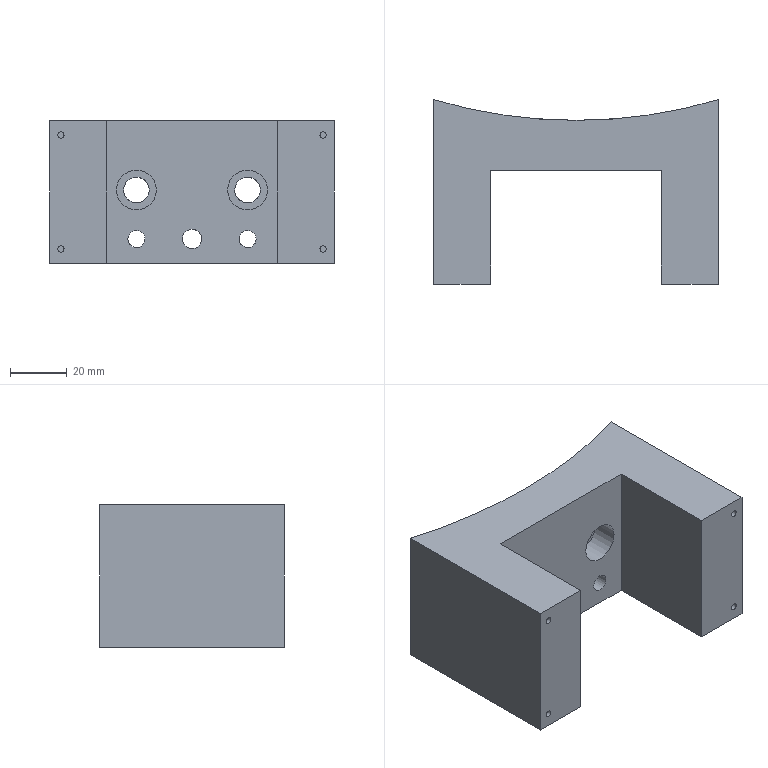Part | NX | 1 solid | 27 faces | box 100 x 64.77 x 50 mm | volume 173660 mm3 | plane 15 | cylinder 12 | commonest cylinder face diameters 2.2 x4 6 x2 9 x2 14 x2 6.8 x1 351 x1
STEP:
#1=CARTESIAN_POINT('',(-50.,32.385,0.));
#2=VERTEX_POINT('',#1);
#3=CARTESIAN_POINT('',(-50.,-32.385,0.));
#4=VERTEX_POINT('',#3);
#5=CARTESIAN_POINT('',(-50.,32.385,0.));
#6=DIRECTION('',(0.,-1.,0.));
#7=VECTOR('',#6,1000.);
#8=LINE('',#5,#7);
#9=EDGE_CURVE('',#2,#4,#8,.T.);
#10=ORIENTED_EDGE('',*,*,#9,.F.);
#11=CARTESIAN_POINT('',(-50.,32.385,-50.));
#12=VERTEX_POINT('',#11);
#13=CARTESIAN_POINT('',(-50.,32.385,-50.));
#14=DIRECTION('',(0.,0.,1.));
#15=VECTOR('',#14,1000.);
#16=LINE('',#13,#15);
#17=EDGE_CURVE('',#12,#2,#16,.T.);
#18=ORIENTED_EDGE('',*,*,#17,.F.);
#19=CARTESIAN_POINT('',(-50.,-32.385,-50.));
#20=VERTEX_POINT('',#19);
#21=CARTESIAN_POINT('',(-50.,32.385,-50.));
#22=DIRECTION('',(0.,-1.,0.));
#23=VECTOR('',#22,1000.);
#24=LINE('',#21,#23);
#25=EDGE_CURVE('',#12,#20,#24,.T.);
#26=ORIENTED_EDGE('',*,*,#25,.T.);
#27=CARTESIAN_POINT('',(-50.,-32.385,-50.));
#28=DIRECTION('',(0.,0.,1.));
#29=VECTOR('',#28,1000.);
#30=LINE('',#27,#29);
#31=EDGE_CURVE('',#20,#4,#30,.T.);
#32=ORIENTED_EDGE('',*,*,#31,.T.);
#33=EDGE_LOOP('',(#10,#18,#26,#32));
#34=FACE_BOUND('',#33,.T.);
#35=CARTESIAN_POINT('',(-50.,32.385,-50.));
#36=DIRECTION('',(-1.,0.,0.));
#37=DIRECTION('',(0.,-1.,0.));
#38=AXIS2_PLACEMENT_3D('',#35,#36,#37);
#39=PLANE('',#38);
#40=ADVANCED_FACE('',(#34),#39,.T.);
#41=CARTESIAN_POINT('',(-44.9,-32.385,-5.));
#42=VERTEX_POINT('',#41);
#43=CARTESIAN_POINT('',(-46.,-32.385,-5.));
#44=DIRECTION('',(0.,1.,0.));
#45=DIRECTION('',(1.,0.,0.));
#46=AXIS2_PLACEMENT_3D('',#43,#44,#45);
#47=CIRCLE('',#46,1.1);
#48=EDGE_CURVE('',#42,#42,#47,.T.);
#49=ORIENTED_EDGE('',*,*,#48,.T.);
#50=EDGE_LOOP('',(#49));
#51=FACE_BOUND('',#50,.T.);
#52=CARTESIAN_POINT('',(-44.9,-32.385,-45.));
#53=VERTEX_POINT('',#52);
#54=CARTESIAN_POINT('',(-46.,-32.385,-45.));
#55=DIRECTION('',(0.,1.,0.));
#56=DIRECTION('',(1.,0.,0.));
#57=AXIS2_PLACEMENT_3D('',#54,#55,#56);
#58=CIRCLE('',#57,1.1);
#59=EDGE_CURVE('',#53,#53,#58,.T.);
#60=ORIENTED_EDGE('',*,*,#59,.T.);
#61=EDGE_LOOP('',(#60));
#62=FACE_BOUND('',#61,.T.);
#63=CARTESIAN_POINT('',(-30.,-32.385,0.));
#64=VERTEX_POINT('',#63);
#65=CARTESIAN_POINT('',(-50.,-32.385,0.));
#66=DIRECTION('',(1.,0.,0.));
#67=VECTOR('',#66,1000.);
#68=LINE('',#65,#67);
#69=EDGE_CURVE('',#4,#64,#68,.T.);
#70=ORIENTED_EDGE('',*,*,#69,.F.);
#71=ORIENTED_EDGE('',*,*,#31,.F.);
#72=CARTESIAN_POINT('',(-30.,-32.385,-50.));
#73=VERTEX_POINT('',#72);
#74=CARTESIAN_POINT('',(-50.,-32.385,-50.));
#75=DIRECTION('',(1.,0.,0.));
#76=VECTOR('',#75,1000.);
#77=LINE('',#74,#76);
#78=EDGE_CURVE('',#20,#73,#77,.T.);
#79=ORIENTED_EDGE('',*,*,#78,.T.);
#80=CARTESIAN_POINT('',(-30.,-32.385,-50.));
#81=DIRECTION('',(0.,0.,1.));
#82=VECTOR('',#81,1000.);
#83=LINE('',#80,#82);
#84=EDGE_CURVE('',#73,#64,#83,.T.);
#85=ORIENTED_EDGE('',*,*,#84,.T.);
#86=EDGE_LOOP('',(#70,#71,#79,#85));
#87=FACE_BOUND('',#86,.T.);
#88=CARTESIAN_POINT('',(-50.,-32.385,-50.));
#89=DIRECTION('',(0.,-1.,0.));
#90=DIRECTION('',(0.,0.,-1.));
#91=AXIS2_PLACEMENT_3D('',#88,#89,#90);
#92=PLANE('',#91);
#93=ADVANCED_FACE('',(#51,#62,#87),#92,.T.);
#94=CARTESIAN_POINT('',(-30.,7.615,0.));
#95=VERTEX_POINT('',#94);
#96=CARTESIAN_POINT('',(-30.,-32.385,0.));
#97=DIRECTION('',(0.,1.,0.));
#98=VECTOR('',#97,1000.);
#99=LINE('',#96,#98);
#100=EDGE_CURVE('',#64,#95,#99,.T.);
#101=ORIENTED_EDGE('',*,*,#100,.F.);
#102=ORIENTED_EDGE('',*,*,#84,.F.);
#103=CARTESIAN_POINT('',(-30.,7.615,-50.));
#104=VERTEX_POINT('',#103);
#105=CARTESIAN_POINT('',(-30.,-32.385,-50.));
#106=DIRECTION('',(0.,1.,0.));
#107=VECTOR('',#106,1000.);
#108=LINE('',#105,#107);
#109=EDGE_CURVE('',#73,#104,#108,.T.);
#110=ORIENTED_EDGE('',*,*,#109,.T.);
#111=CARTESIAN_POINT('',(-30.,7.615,-50.));
#112=DIRECTION('',(0.,0.,1.));
#113=VECTOR('',#112,1000.);
#114=LINE('',#111,#113);
#115=EDGE_CURVE('',#104,#95,#114,.T.);
#116=ORIENTED_EDGE('',*,*,#115,.T.);
#117=EDGE_LOOP('',(#101,#102,#110,#116));
#118=FACE_BOUND('',#117,.T.);
#119=CARTESIAN_POINT('',(-30.,-32.385,-50.));
#120=DIRECTION('',(1.,0.,0.));
#121=DIRECTION('',(0.,1.,0.));
#122=AXIS2_PLACEMENT_3D('',#119,#120,#121);
#123=PLANE('',#122);
#124=ADVANCED_FACE('',(#118),#123,.T.);
#125=CARTESIAN_POINT('',(26.5,7.615,-24.3));
#126=VERTEX_POINT('',#125);
#127=CARTESIAN_POINT('',(19.5,7.615,-24.3));
#128=DIRECTION('',(0.,1.,0.));
#129=DIRECTION('',(1.,0.,0.));
#130=AXIS2_PLACEMENT_3D('',#127,#128,#129);
#131=CIRCLE('',#130,7.);
#132=EDGE_CURVE('',#126,#126,#131,.T.);
#133=ORIENTED_EDGE('',*,*,#132,.T.);
#134=EDGE_LOOP('',(#133));
#135=FACE_BOUND('',#134,.T.);
#136=CARTESIAN_POINT('',(-12.5,7.615,-24.3));
#137=VERTEX_POINT('',#136);
#138=CARTESIAN_POINT('',(-19.5,7.615,-24.3));
#139=DIRECTION('',(0.,1.,0.));
#140=DIRECTION('',(1.,0.,0.));
#141=AXIS2_PLACEMENT_3D('',#138,#139,#140);
#142=CIRCLE('',#141,7.);
#143=EDGE_CURVE('',#137,#137,#142,.T.);
#144=ORIENTED_EDGE('',*,*,#143,.T.);
#145=EDGE_LOOP('',(#144));
#146=FACE_BOUND('',#145,.T.);
#147=CARTESIAN_POINT('',(-16.5,7.615,-41.5));
#148=VERTEX_POINT('',#147);
#149=CARTESIAN_POINT('',(-19.5,7.615,-41.5));
#150=DIRECTION('',(0.,-1.,0.));
#151=DIRECTION('',(1.,0.,0.));
#152=AXIS2_PLACEMENT_3D('',#149,#150,#151);
#153=CIRCLE('',#152,3.);
#154=EDGE_CURVE('',#148,#148,#153,.T.);
#155=ORIENTED_EDGE('',*,*,#154,.F.);
#156=EDGE_LOOP('',(#155));
#157=FACE_BOUND('',#156,.T.);
#158=CARTESIAN_POINT('',(3.4,7.615,-41.5));
#159=VERTEX_POINT('',#158);
#160=CARTESIAN_POINT('',(0.,7.615,-41.5));
#161=DIRECTION('',(0.,-1.,0.));
#162=DIRECTION('',(1.,0.,0.));
#163=AXIS2_PLACEMENT_3D('',#160,#161,#162);
#164=CIRCLE('',#163,3.4);
#165=EDGE_CURVE('',#159,#159,#164,.T.);
#166=ORIENTED_EDGE('',*,*,#165,.F.);
#167=EDGE_LOOP('',(#166));
#168=FACE_BOUND('',#167,.T.);
#169=CARTESIAN_POINT('',(22.5,7.615,-41.5));
#170=VERTEX_POINT('',#169);
#171=CARTESIAN_POINT('',(19.5,7.615,-41.5));
#172=DIRECTION('',(0.,-1.,0.));
#173=DIRECTION('',(1.,0.,0.));
#174=AXIS2_PLACEMENT_3D('',#171,#172,#173);
#175=CIRCLE('',#174,3.);
#176=EDGE_CURVE('',#170,#170,#175,.T.);
#177=ORIENTED_EDGE('',*,*,#176,.F.);
#178=EDGE_LOOP('',(#177));
#179=FACE_BOUND('',#178,.T.);
#180=CARTESIAN_POINT('',(30.,7.615,0.));
#181=VERTEX_POINT('',#180);
#182=CARTESIAN_POINT('',(-30.,7.615,0.));
#183=DIRECTION('',(1.,0.,0.));
#184=VECTOR('',#183,1000.);
#185=LINE('',#182,#184);
#186=EDGE_CURVE('',#95,#181,#185,.T.);
#187=ORIENTED_EDGE('',*,*,#186,.F.);
#188=ORIENTED_EDGE('',*,*,#115,.F.);
#189=CARTESIAN_POINT('',(30.,7.615,-50.));
#190=VERTEX_POINT('',#189);
#191=CARTESIAN_POINT('',(-30.,7.615,-50.));
#192=DIRECTION('',(1.,0.,0.));
#193=VECTOR('',#192,1000.);
#194=LINE('',#191,#193);
#195=EDGE_CURVE('',#104,#190,#194,.T.);
#196=ORIENTED_EDGE('',*,*,#195,.T.);
#197=CARTESIAN_POINT('',(30.,7.615,-50.));
#198=DIRECTION('',(0.,0.,1.));
#199=VECTOR('',#198,1000.);
#200=LINE('',#197,#199);
#201=EDGE_CURVE('',#190,#181,#200,.T.);
#202=ORIENTED_EDGE('',*,*,#201,.T.);
#203=EDGE_LOOP('',(#187,#188,#196,#202));
#204=FACE_BOUND('',#203,.T.);
#205=CARTESIAN_POINT('',(-30.,7.615,-50.));
#206=DIRECTION('',(0.,-1.,0.));
#207=DIRECTION('',(1.,0.,0.));
#208=AXIS2_PLACEMENT_3D('',#205,#206,#207);
#209=PLANE('',#208);
#210=ADVANCED_FACE('',(#135,#146,#157,#168,#179,#204),#209,.T.);
#211=CARTESIAN_POINT('',(30.,-32.385,0.));
#212=VERTEX_POINT('',#211);
#213=CARTESIAN_POINT('',(30.,7.615,0.));
#214=DIRECTION('',(0.,-1.,0.));
#215=VECTOR('',#214,1000.);
#216=LINE('',#213,#215);
#217=EDGE_CURVE('',#181,#212,#216,.T.);
#218=ORIENTED_EDGE('',*,*,#217,.F.);
#219=ORIENTED_EDGE('',*,*,#201,.F.);
#220=CARTESIAN_POINT('',(30.,-32.385,-50.));
#221=VERTEX_POINT('',#220);
#222=CARTESIAN_POINT('',(30.,7.615,-50.));
#223=DIRECTION('',(0.,-1.,0.));
#224=VECTOR('',#223,1000.);
#225=LINE('',#222,#224);
#226=EDGE_CURVE('',#190,#221,#225,.T.);
#227=ORIENTED_EDGE('',*,*,#226,.T.);
#228=CARTESIAN_POINT('',(30.,-32.385,-50.));
#229=DIRECTION('',(0.,0.,1.));
#230=VECTOR('',#229,1000.);
#231=LINE('',#228,#230);
#232=EDGE_CURVE('',#221,#212,#231,.T.);
#233=ORIENTED_EDGE('',*,*,#232,.T.);
#234=EDGE_LOOP('',(#218,#219,#227,#233));
#235=FACE_BOUND('',#234,.T.);
#236=CARTESIAN_POINT('',(30.,7.615,-50.));
#237=DIRECTION('',(-1.,0.,0.));
#238=DIRECTION('',(0.,-1.,0.));
#239=AXIS2_PLACEMENT_3D('',#236,#237,#238);
#240=PLANE('',#239);
#241=ADVANCED_FACE('',(#235),#240,.T.);
#242=CARTESIAN_POINT('',(47.1,-32.385,-45.));
#243=VERTEX_POINT('',#242);
#244=CARTESIAN_POINT('',(46.,-32.385,-45.));
#245=DIRECTION('',(0.,1.,0.));
#246=DIRECTION('',(1.,0.,0.));
#247=AXIS2_PLACEMENT_3D('',#244,#245,#246);
#248=CIRCLE('',#247,1.1);
#249=EDGE_CURVE('',#243,#243,#248,.T.);
#250=ORIENTED_EDGE('',*,*,#249,.T.);
#251=EDGE_LOOP('',(#250));
#252=FACE_BOUND('',#251,.T.);
#253=CARTESIAN_POINT('',(47.1,-32.385,-5.));
#254=VERTEX_POINT('',#253);
#255=CARTESIAN_POINT('',(46.,-32.385,-5.));
#256=DIRECTION('',(0.,1.,0.));
#257=DIRECTION('',(1.,0.,0.));
#258=AXIS2_PLACEMENT_3D('',#255,#256,#257);
#259=CIRCLE('',#258,1.1);
#260=EDGE_CURVE('',#254,#254,#259,.T.);
#261=ORIENTED_EDGE('',*,*,#260,.T.);
#262=EDGE_LOOP('',(#261));
#263=FACE_BOUND('',#262,.T.);
#264=CARTESIAN_POINT('',(50.,-32.385,0.));
#265=VERTEX_POINT('',#264);
#266=CARTESIAN_POINT('',(30.,-32.385,0.));
#267=DIRECTION('',(1.,0.,0.));
#268=VECTOR('',#267,1000.);
#269=LINE('',#266,#268);
#270=EDGE_CURVE('',#212,#265,#269,.T.);
#271=ORIENTED_EDGE('',*,*,#270,.F.);
#272=ORIENTED_EDGE('',*,*,#232,.F.);
#273=CARTESIAN_POINT('',(50.,-32.385,-50.));
#274=VERTEX_POINT('',#273);
#275=CARTESIAN_POINT('',(30.,-32.385,-50.));
#276=DIRECTION('',(1.,0.,0.));
#277=VECTOR('',#276,1000.);
#278=LINE('',#275,#277);
#279=EDGE_CURVE('',#221,#274,#278,.T.);
#280=ORIENTED_EDGE('',*,*,#279,.T.);
#281=CARTESIAN_POINT('',(50.,-32.385,-50.));
#282=DIRECTION('',(0.,0.,1.));
#283=VECTOR('',#282,1000.);
#284=LINE('',#281,#283);
#285=EDGE_CURVE('',#274,#265,#284,.T.);
#286=ORIENTED_EDGE('',*,*,#285,.T.);
#287=EDGE_LOOP('',(#271,#272,#280,#286));
#288=FACE_BOUND('',#287,.T.);
#289=CARTESIAN_POINT('',(30.,-32.385,-50.));
#290=DIRECTION('',(0.,-1.,0.));
#291=DIRECTION('',(0.,0.,-1.));
#292=AXIS2_PLACEMENT_3D('',#289,#290,#291);
#293=PLANE('',#292);
#294=ADVANCED_FACE('',(#252,#263,#288),#293,.T.);
#295=CARTESIAN_POINT('',(50.,32.385,0.));
#296=VERTEX_POINT('',#295);
#297=CARTESIAN_POINT('',(50.,-32.385,0.));
#298=DIRECTION('',(0.,1.,0.));
#299=VECTOR('',#298,1000.);
#300=LINE('',#297,#299);
#301=EDGE_CURVE('',#265,#296,#300,.T.);
#302=ORIENTED_EDGE('',*,*,#301,.F.);
#303=ORIENTED_EDGE('',*,*,#285,.F.);
#304=CARTESIAN_POINT('',(50.,32.385,-50.));
#305=VERTEX_POINT('',#304);
#306=CARTESIAN_POINT('',(50.,-32.385,-50.));
#307=DIRECTION('',(0.,1.,0.));
#308=VECTOR('',#307,1000.);
#309=LINE('',#306,#308);
#310=EDGE_CURVE('',#274,#305,#309,.T.);
#311=ORIENTED_EDGE('',*,*,#310,.T.);
#312=CARTESIAN_POINT('',(50.,32.385,-50.));
#313=DIRECTION('',(0.,0.,1.));
#314=VECTOR('',#313,1000.);
#315=LINE('',#312,#314);
#316=EDGE_CURVE('',#305,#296,#315,.T.);
#317=ORIENTED_EDGE('',*,*,#316,.T.);
#318=EDGE_LOOP('',(#302,#303,#311,#317));
#319=FACE_BOUND('',#318,.T.);
#320=CARTESIAN_POINT('',(50.,-32.385,-50.));
#321=DIRECTION('',(1.,0.,0.));
#322=DIRECTION('',(0.,1.,0.));
#323=AXIS2_PLACEMENT_3D('',#320,#321,#322);
#324=PLANE('',#323);
#325=ADVANCED_FACE('',(#319),#324,.T.);
#326=CARTESIAN_POINT('',(-19.5,26.198,-19.8));
#327=VERTEX_POINT('',#326);
#328=CARTESIAN_POINT('',(-23.019,26.621,-20.766));
#329=CARTESIAN_POINT('',(-19.501,26.184,-19.316));
#330=CARTESIAN_POINT('',(-15.979,25.834,-20.769));
#331=CARTESIAN_POINT('',(-14.51,25.714,-24.301));
#332=CARTESIAN_POINT('',(-15.983,25.834,-27.838));
#333=CARTESIAN_POINT('',(-19.511,26.185,-29.282));
#334=CARTESIAN_POINT('',(-23.016,26.621,-27.833));
#335=CARTESIAN_POINT('',(-24.491,26.83,-24.302));
#336=CARTESIAN_POINT('',(-23.019,26.621,-20.766));
#337=CARTESIAN_POINT('',(-19.501,26.184,-19.316));
#338=CARTESIAN_POINT('',(-15.979,25.834,-20.769));
#339=B_SPLINE_CURVE_WITH_KNOTS('',3,(#328,#329,#330,#331,#332,#333,#334,#335,#336,#337,#338),.UNSPECIFIED.,.T.,.F.,(1,1,1,1,1,1,1,1,1,1,1,1,1,1,1),(-0.01058,-0.007056,-0.003528,0.,0.003528,0.007056,0.01058,0.01411,0.01764,0.02117,0.02469,0.02822,0.03175,0.03528,0.03881),.UNSPECIFIED.);
#340=EDGE_CURVE('',#327,#327,#339,.T.);
#341=ORIENTED_EDGE('',*,*,#340,.F.);
#342=EDGE_LOOP('',(#341));
#343=FACE_BOUND('',#342,.T.);
#344=CARTESIAN_POINT('',(-19.5,26.198,-38.5));
#345=VERTEX_POINT('',#344);
#346=CARTESIAN_POINT('',(-21.846,26.474,-39.145));
#347=CARTESIAN_POINT('',(-19.5,26.192,-38.178));
#348=CARTESIAN_POINT('',(-17.153,25.949,-39.145));
#349=CARTESIAN_POINT('',(-16.173,25.859,-41.499));
#350=CARTESIAN_POINT('',(-17.155,25.949,-43.858));
#351=CARTESIAN_POINT('',(-19.505,26.193,-44.821));
#352=CARTESIAN_POINT('',(-21.844,26.473,-43.857));
#353=CARTESIAN_POINT('',(-22.827,26.603,-41.502));
#354=CARTESIAN_POINT('',(-21.846,26.474,-39.145));
#355=CARTESIAN_POINT('',(-19.5,26.192,-38.178));
#356=CARTESIAN_POINT('',(-17.153,25.949,-39.145));
#357=B_SPLINE_CURVE_WITH_KNOTS('',3,(#346,#347,#348,#349,#350,#351,#352,#353,#354,#355,#356),.UNSPECIFIED.,.T.,.F.,(1,1,1,1,1,1,1,1,1,1,1,1,1,1,1),(-0.007055,-0.004704,-0.002352,0.,0.002352,0.004704,0.007055,0.009407,0.01176,0.01411,0.01646,0.01881,0.02117,0.02352,0.02587),.UNSPECIFIED.);
#358=EDGE_CURVE('',#345,#345,#357,.T.);
#359=ORIENTED_EDGE('',*,*,#358,.F.);
#360=EDGE_LOOP('',(#359));
#361=FACE_BOUND('',#360,.T.);
#362=CARTESIAN_POINT('',(0.,25.112,-38.1));
#363=VERTEX_POINT('',#362);
#364=CARTESIAN_POINT('',(-2.667,25.128,-38.838));
#365=CARTESIAN_POINT('',(0.0006847,25.104,-37.731));
#366=CARTESIAN_POINT('',(2.665,25.128,-38.837));
#367=CARTESIAN_POINT('',(3.767,25.153,-41.497));
#368=CARTESIAN_POINT('',(2.666,25.128,-44.163));
#369=CARTESIAN_POINT('',(0.0004927,25.104,-45.267));
#370=CARTESIAN_POINT('',(-2.661,25.128,-44.167));
#371=CARTESIAN_POINT('',(-3.768,25.153,-41.504));
#372=CARTESIAN_POINT('',(-2.667,25.128,-38.838));
#373=CARTESIAN_POINT('',(0.0006847,25.104,-37.731));
#374=CARTESIAN_POINT('',(2.665,25.128,-38.837));
#375=B_SPLINE_CURVE_WITH_KNOTS('',3,(#364,#365,#366,#367,#368,#369,#370,#371,#372,#373,#374),.UNSPECIFIED.,.T.,.F.,(1,1,1,1,1,1,1,1,1,1,1,1,1,1,1),(-0.007972,-0.005315,-0.002657,0.,0.002657,0.005315,0.007972,0.01063,0.01329,0.01594,0.0186,0.02126,0.02392,0.02657,0.02923),.UNSPECIFIED.);
#376=EDGE_CURVE('',#363,#363,#375,.T.);
#377=ORIENTED_EDGE('',*,*,#376,.F.);
#378=EDGE_LOOP('',(#377));
#379=FACE_BOUND('',#378,.T.);
#380=CARTESIAN_POINT('',(19.5,26.198,-19.8));
#381=VERTEX_POINT('',#380);
#382=CARTESIAN_POINT('',(15.975,25.834,-20.77));
#383=CARTESIAN_POINT('',(19.503,26.184,-19.316));
#384=CARTESIAN_POINT('',(23.014,26.621,-20.765));
#385=CARTESIAN_POINT('',(24.49,26.83,-24.291));
#386=CARTESIAN_POINT('',(23.024,26.622,-27.828));
#387=CARTESIAN_POINT('',(19.512,26.185,-29.282));
#388=CARTESIAN_POINT('',(15.991,25.835,-27.843));
#389=CARTESIAN_POINT('',(14.509,25.714,-24.311));
#390=CARTESIAN_POINT('',(15.975,25.834,-20.77));
#391=CARTESIAN_POINT('',(19.503,26.184,-19.316));
#392=CARTESIAN_POINT('',(23.014,26.621,-20.765));
#393=B_SPLINE_CURVE_WITH_KNOTS('',3,(#382,#383,#384,#385,#386,#387,#388,#389,#390,#391,#392),.UNSPECIFIED.,.T.,.F.,(1,1,1,1,1,1,1,1,1,1,1,1,1,1,1),(-0.01058,-0.007055,-0.003528,0.,0.003528,0.007055,0.01058,0.01411,0.01764,0.02117,0.02469,0.02822,0.03175,0.03528,0.0388),.UNSPECIFIED.);
#394=EDGE_CURVE('',#381,#381,#393,.T.);
#395=ORIENTED_EDGE('',*,*,#394,.F.);
#396=EDGE_LOOP('',(#395));
#397=FACE_BOUND('',#396,.T.);
#398=CARTESIAN_POINT('',(19.5,26.198,-38.5));
#399=VERTEX_POINT('',#398);
#400=CARTESIAN_POINT('',(17.15,25.949,-39.146));
#401=CARTESIAN_POINT('',(19.501,26.192,-38.178));
#402=CARTESIAN_POINT('',(21.844,26.473,-39.144));
#403=CARTESIAN_POINT('',(22.827,26.603,-41.495));
#404=CARTESIAN_POINT('',(21.848,26.474,-43.853));
#405=CARTESIAN_POINT('',(19.505,26.193,-44.821));
#406=CARTESIAN_POINT('',(17.16,25.95,-43.861));
#407=CARTESIAN_POINT('',(16.172,25.859,-41.506));
#408=CARTESIAN_POINT('',(17.15,25.949,-39.146));
#409=CARTESIAN_POINT('',(19.501,26.192,-38.178));
#410=CARTESIAN_POINT('',(21.844,26.473,-39.144));
#411=B_SPLINE_CURVE_WITH_KNOTS('',3,(#400,#401,#402,#403,#404,#405,#406,#407,#408,#409,#410),.UNSPECIFIED.,.T.,.F.,(1,1,1,1,1,1,1,1,1,1,1,1,1,1,1),(-0.007055,-0.004704,-0.002352,0.,0.002352,0.004704,0.007055,0.009407,0.01176,0.01411,0.01646,0.01881,0.02117,0.02352,0.02587),.UNSPECIFIED.);
#412=EDGE_CURVE('',#399,#399,#411,.T.);
#413=ORIENTED_EDGE('',*,*,#412,.F.);
#414=EDGE_LOOP('',(#413));
#415=FACE_BOUND('',#414,.T.);
#416=CARTESIAN_POINT('',(0.,200.612,0.));
#417=DIRECTION('',(0.,0.,-1.));
#418=DIRECTION('',(1.,0.,0.));
#419=AXIS2_PLACEMENT_3D('',#416,#417,#418);
#420=CIRCLE('',#419,175.5);
#421=EDGE_CURVE('',#296,#2,#420,.T.);
#422=ORIENTED_EDGE('',*,*,#421,.F.);
#423=ORIENTED_EDGE('',*,*,#316,.F.);
#424=CARTESIAN_POINT('',(0.,200.612,-50.));
#425=DIRECTION('',(0.,0.,-1.));
#426=DIRECTION('',(1.,0.,0.));
#427=AXIS2_PLACEMENT_3D('',#424,#425,#426);
#428=CIRCLE('',#427,175.5);
#429=EDGE_CURVE('',#305,#12,#428,.T.);
#430=ORIENTED_EDGE('',*,*,#429,.T.);
#431=ORIENTED_EDGE('',*,*,#17,.T.);
#432=EDGE_LOOP('',(#422,#423,#430,#431));
#433=FACE_BOUND('',#432,.T.);
#434=CARTESIAN_POINT('',(0.,200.612,-50.));
#435=DIRECTION('',(0.,0.,1.));
#436=DIRECTION('',(1.,0.,0.));
#437=AXIS2_PLACEMENT_3D('',#434,#435,#436);
#438=CYLINDRICAL_SURFACE('',#437,175.5);
#439=ADVANCED_FACE('',(#343,#361,#379,#397,#415,#433),#438,.F.);
#440=ORIENTED_EDGE('',*,*,#25,.F.);
#441=ORIENTED_EDGE('',*,*,#429,.F.);
#442=ORIENTED_EDGE('',*,*,#310,.F.);
#443=ORIENTED_EDGE('',*,*,#279,.F.);
#444=ORIENTED_EDGE('',*,*,#226,.F.);
#445=ORIENTED_EDGE('',*,*,#195,.F.);
#446=ORIENTED_EDGE('',*,*,#109,.F.);
#447=ORIENTED_EDGE('',*,*,#78,.F.);
#448=EDGE_LOOP('',(#440,#441,#442,#443,#444,#445,#446,#447));
#449=FACE_BOUND('',#448,.T.);
#450=CARTESIAN_POINT('',(0.,200.612,-50.));
#451=DIRECTION('',(0.,0.,-1.));
#452=DIRECTION('',(-1.,0.,0.));
#453=AXIS2_PLACEMENT_3D('',#450,#451,#452);
#454=PLANE('',#453);
#455=ADVANCED_FACE('',(#449),#454,.T.);
#456=ORIENTED_EDGE('',*,*,#9,.T.);
#457=ORIENTED_EDGE('',*,*,#69,.T.);
#458=ORIENTED_EDGE('',*,*,#100,.T.);
#459=ORIENTED_EDGE('',*,*,#186,.T.);
#460=ORIENTED_EDGE('',*,*,#217,.T.);
#461=ORIENTED_EDGE('',*,*,#270,.T.);
#462=ORIENTED_EDGE('',*,*,#301,.T.);
#463=ORIENTED_EDGE('',*,*,#421,.T.);
#464=EDGE_LOOP('',(#456,#457,#458,#459,#460,#461,#462,#463));
#465=FACE_BOUND('',#464,.T.);
#466=CARTESIAN_POINT('',(0.,200.612,0.));
#467=DIRECTION('',(0.,0.,-1.));
#468=DIRECTION('',(-1.,0.,0.));
#469=AXIS2_PLACEMENT_3D('',#466,#467,#468);
#470=PLANE('',#469);
#471=ADVANCED_FACE('',(#465),#470,.F.);
#472=ORIENTED_EDGE('',*,*,#260,.F.);
#473=EDGE_LOOP('',(#472));
#474=FACE_BOUND('',#473,.T.);
#475=CARTESIAN_POINT('',(47.1,-21.385,-5.));
#476=VERTEX_POINT('',#475);
#477=CARTESIAN_POINT('',(46.,-21.385,-5.));
#478=DIRECTION('',(0.,1.,0.));
#479=DIRECTION('',(1.,0.,0.));
#480=AXIS2_PLACEMENT_3D('',#477,#478,#479);
#481=CIRCLE('',#480,1.1);
#482=EDGE_CURVE('',#476,#476,#481,.F.);
#483=ORIENTED_EDGE('',*,*,#482,.F.);
#484=EDGE_LOOP('',(#483));
#485=FACE_BOUND('',#484,.T.);
#486=CARTESIAN_POINT('',(46.,-32.385,-5.));
#487=DIRECTION('',(0.,1.,0.));
#488=DIRECTION('',(0.,0.,1.));
#489=AXIS2_PLACEMENT_3D('',#486,#487,#488);
#490=CYLINDRICAL_SURFACE('',#489,1.1);
#491=ADVANCED_FACE('',(#474,#485),#490,.F.);
#492=ORIENTED_EDGE('',*,*,#482,.T.);
#493=EDGE_LOOP('',(#492));
#494=FACE_BOUND('',#493,.T.);
#495=CARTESIAN_POINT('',(46.,-21.385,-5.));
#496=DIRECTION('',(0.,1.,0.));
#497=DIRECTION('',(0.,0.,1.));
#498=AXIS2_PLACEMENT_3D('',#495,#496,#497);
#499=PLANE('',#498);
#500=ADVANCED_FACE('',(#494),#499,.F.);
#501=ORIENTED_EDGE('',*,*,#249,.F.);
#502=EDGE_LOOP('',(#501));
#503=FACE_BOUND('',#502,.T.);
#504=CARTESIAN_POINT('',(47.1,-21.385,-45.));
#505=VERTEX_POINT('',#504);
#506=CARTESIAN_POINT('',(46.,-21.385,-45.));
#507=DIRECTION('',(0.,1.,0.));
#508=DIRECTION('',(1.,0.,0.));
#509=AXIS2_PLACEMENT_3D('',#506,#507,#508);
#510=CIRCLE('',#509,1.1);
#511=EDGE_CURVE('',#505,#505,#510,.F.);
#512=ORIENTED_EDGE('',*,*,#511,.F.);
#513=EDGE_LOOP('',(#512));
#514=FACE_BOUND('',#513,.T.);
#515=CARTESIAN_POINT('',(46.,-32.385,-45.));
#516=DIRECTION('',(0.,1.,0.));
#517=DIRECTION('',(0.,0.,1.));
#518=AXIS2_PLACEMENT_3D('',#515,#516,#517);
#519=CYLINDRICAL_SURFACE('',#518,1.1);
#520=ADVANCED_FACE('',(#503,#514),#519,.F.);
#521=ORIENTED_EDGE('',*,*,#511,.T.);
#522=EDGE_LOOP('',(#521));
#523=FACE_BOUND('',#522,.T.);
#524=CARTESIAN_POINT('',(46.,-21.385,-45.));
#525=DIRECTION('',(0.,1.,0.));
#526=DIRECTION('',(0.,0.,1.));
#527=AXIS2_PLACEMENT_3D('',#524,#525,#526);
#528=PLANE('',#527);
#529=ADVANCED_FACE('',(#523),#528,.F.);
#530=ORIENTED_EDGE('',*,*,#59,.F.);
#531=EDGE_LOOP('',(#530));
#532=FACE_BOUND('',#531,.T.);
#533=CARTESIAN_POINT('',(-44.9,-21.385,-45.));
#534=VERTEX_POINT('',#533);
#535=CARTESIAN_POINT('',(-46.,-21.385,-45.));
#536=DIRECTION('',(0.,1.,0.));
#537=DIRECTION('',(1.,0.,0.));
#538=AXIS2_PLACEMENT_3D('',#535,#536,#537);
#539=CIRCLE('',#538,1.1);
#540=EDGE_CURVE('',#534,#534,#539,.F.);
#541=ORIENTED_EDGE('',*,*,#540,.F.);
#542=EDGE_LOOP('',(#541));
#543=FACE_BOUND('',#542,.T.);
#544=CARTESIAN_POINT('',(-46.,-32.385,-45.));
#545=DIRECTION('',(0.,1.,0.));
#546=DIRECTION('',(0.,0.,1.));
#547=AXIS2_PLACEMENT_3D('',#544,#545,#546);
#548=CYLINDRICAL_SURFACE('',#547,1.1);
#549=ADVANCED_FACE('',(#532,#543),#548,.F.);
#550=ORIENTED_EDGE('',*,*,#540,.T.);
#551=EDGE_LOOP('',(#550));
#552=FACE_BOUND('',#551,.T.);
#553=CARTESIAN_POINT('',(-46.,-21.385,-45.));
#554=DIRECTION('',(0.,1.,0.));
#555=DIRECTION('',(0.,0.,1.));
#556=AXIS2_PLACEMENT_3D('',#553,#554,#555);
#557=PLANE('',#556);
#558=ADVANCED_FACE('',(#552),#557,.F.);
#559=ORIENTED_EDGE('',*,*,#48,.F.);
#560=EDGE_LOOP('',(#559));
#561=FACE_BOUND('',#560,.T.);
#562=CARTESIAN_POINT('',(-44.9,-21.385,-5.));
#563=VERTEX_POINT('',#562);
#564=CARTESIAN_POINT('',(-46.,-21.385,-5.));
#565=DIRECTION('',(0.,1.,0.));
#566=DIRECTION('',(1.,0.,0.));
#567=AXIS2_PLACEMENT_3D('',#564,#565,#566);
#568=CIRCLE('',#567,1.1);
#569=EDGE_CURVE('',#563,#563,#568,.F.);
#570=ORIENTED_EDGE('',*,*,#569,.F.);
#571=EDGE_LOOP('',(#570));
#572=FACE_BOUND('',#571,.T.);
#573=CARTESIAN_POINT('',(-46.,-32.385,-5.));
#574=DIRECTION('',(0.,1.,0.));
#575=DIRECTION('',(0.,0.,1.));
#576=AXIS2_PLACEMENT_3D('',#573,#574,#575);
#577=CYLINDRICAL_SURFACE('',#576,1.1);
#578=ADVANCED_FACE('',(#561,#572),#577,.F.);
#579=ORIENTED_EDGE('',*,*,#569,.T.);
#580=EDGE_LOOP('',(#579));
#581=FACE_BOUND('',#580,.T.);
#582=CARTESIAN_POINT('',(-46.,-21.385,-5.));
#583=DIRECTION('',(0.,1.,0.));
#584=DIRECTION('',(0.,0.,1.));
#585=AXIS2_PLACEMENT_3D('',#582,#583,#584);
#586=PLANE('',#585);
#587=ADVANCED_FACE('',(#581),#586,.F.);
#588=ORIENTED_EDGE('',*,*,#176,.T.);
#589=EDGE_LOOP('',(#588));
#590=FACE_BOUND('',#589,.T.);
#591=ORIENTED_EDGE('',*,*,#412,.T.);
#592=EDGE_LOOP('',(#591));
#593=FACE_BOUND('',#592,.T.);
#594=CARTESIAN_POINT('',(19.5,-32.385,-41.5));
#595=DIRECTION('',(0.,1.,0.));
#596=DIRECTION('',(0.,0.,1.));
#597=AXIS2_PLACEMENT_3D('',#594,#595,#596);
#598=CYLINDRICAL_SURFACE('',#597,3.);
#599=ADVANCED_FACE('',(#590,#593),#598,.F.);
#600=CARTESIAN_POINT('',(24.,16.615,-24.3));
#601=VERTEX_POINT('',#600);
#602=CARTESIAN_POINT('',(19.5,16.615,-24.3));
#603=DIRECTION('',(0.,1.,0.));
#604=DIRECTION('',(1.,0.,0.));
#605=AXIS2_PLACEMENT_3D('',#602,#603,#604);
#606=CIRCLE('',#605,4.5);
#607=EDGE_CURVE('',#601,#601,#606,.T.);
#608=ORIENTED_EDGE('',*,*,#607,.F.);
#609=EDGE_LOOP('',(#608));
#610=FACE_BOUND('',#609,.T.);
#611=ORIENTED_EDGE('',*,*,#394,.T.);
#612=EDGE_LOOP('',(#611));
#613=FACE_BOUND('',#612,.T.);
#614=CARTESIAN_POINT('',(19.5,-32.385,-24.3));
#615=DIRECTION('',(0.,1.,0.));
#616=DIRECTION('',(0.,0.,1.));
#617=AXIS2_PLACEMENT_3D('',#614,#615,#616);
#618=CYLINDRICAL_SURFACE('',#617,4.5);
#619=ADVANCED_FACE('',(#610,#613),#618,.F.);
#620=ORIENTED_EDGE('',*,*,#165,.T.);
#621=EDGE_LOOP('',(#620));
#622=FACE_BOUND('',#621,.T.);
#623=ORIENTED_EDGE('',*,*,#376,.T.);
#624=EDGE_LOOP('',(#623));
#625=FACE_BOUND('',#624,.T.);
#626=CARTESIAN_POINT('',(0.,-32.385,-41.5));
#627=DIRECTION('',(0.,1.,0.));
#628=DIRECTION('',(0.,0.,1.));
#629=AXIS2_PLACEMENT_3D('',#626,#627,#628);
#630=CYLINDRICAL_SURFACE('',#629,3.4);
#631=ADVANCED_FACE('',(#622,#625),#630,.F.);
#632=ORIENTED_EDGE('',*,*,#154,.T.);
#633=EDGE_LOOP('',(#632));
#634=FACE_BOUND('',#633,.T.);
#635=ORIENTED_EDGE('',*,*,#358,.T.);
#636=EDGE_LOOP('',(#635));
#637=FACE_BOUND('',#636,.T.);
#638=CARTESIAN_POINT('',(-19.5,-32.385,-41.5));
#639=DIRECTION('',(0.,1.,0.));
#640=DIRECTION('',(0.,0.,1.));
#641=AXIS2_PLACEMENT_3D('',#638,#639,#640);
#642=CYLINDRICAL_SURFACE('',#641,3.);
#643=ADVANCED_FACE('',(#634,#637),#642,.F.);
#644=CARTESIAN_POINT('',(-15.,16.615,-24.3));
#645=VERTEX_POINT('',#644);
#646=CARTESIAN_POINT('',(-19.5,16.615,-24.3));
#647=DIRECTION('',(0.,1.,0.));
#648=DIRECTION('',(1.,0.,0.));
#649=AXIS2_PLACEMENT_3D('',#646,#647,#648);
#650=CIRCLE('',#649,4.5);
#651=EDGE_CURVE('',#645,#645,#650,.T.);
#652=ORIENTED_EDGE('',*,*,#651,.F.);
#653=EDGE_LOOP('',(#652));
#654=FACE_BOUND('',#653,.T.);
#655=ORIENTED_EDGE('',*,*,#340,.T.);
#656=EDGE_LOOP('',(#655));
#657=FACE_BOUND('',#656,.T.);
#658=CARTESIAN_POINT('',(-19.5,-32.385,-24.3));
#659=DIRECTION('',(0.,1.,0.));
#660=DIRECTION('',(0.,0.,1.));
#661=AXIS2_PLACEMENT_3D('',#658,#659,#660);
#662=CYLINDRICAL_SURFACE('',#661,4.5);
#663=ADVANCED_FACE('',(#654,#657),#662,.F.);
#664=ORIENTED_EDGE('',*,*,#143,.F.);
#665=EDGE_LOOP('',(#664));
#666=FACE_BOUND('',#665,.T.);
#667=CARTESIAN_POINT('',(-12.5,16.615,-24.3));
#668=VERTEX_POINT('',#667);
#669=CARTESIAN_POINT('',(-19.5,16.615,-24.3));
#670=DIRECTION('',(0.,1.,0.));
#671=DIRECTION('',(1.,0.,0.));
#672=AXIS2_PLACEMENT_3D('',#669,#670,#671);
#673=CIRCLE('',#672,7.);
#674=EDGE_CURVE('',#668,#668,#673,.F.);
#675=ORIENTED_EDGE('',*,*,#674,.F.);
#676=EDGE_LOOP('',(#675));
#677=FACE_BOUND('',#676,.T.);
#678=CARTESIAN_POINT('',(-19.5,7.615,-24.3));
#679=DIRECTION('',(0.,1.,0.));
#680=DIRECTION('',(0.,0.,1.));
#681=AXIS2_PLACEMENT_3D('',#678,#679,#680);
#682=CYLINDRICAL_SURFACE('',#681,7.);
#683=ADVANCED_FACE('',(#666,#677),#682,.F.);
#684=ORIENTED_EDGE('',*,*,#674,.T.);
#685=EDGE_LOOP('',(#684));
#686=FACE_BOUND('',#685,.T.);
#687=ORIENTED_EDGE('',*,*,#651,.T.);
#688=EDGE_LOOP('',(#687));
#689=FACE_BOUND('',#688,.T.);
#690=CARTESIAN_POINT('',(-19.5,16.615,-24.3));
#691=DIRECTION('',(0.,1.,0.));
#692=DIRECTION('',(0.,0.,1.));
#693=AXIS2_PLACEMENT_3D('',#690,#691,#692);
#694=PLANE('',#693);
#695=ADVANCED_FACE('',(#686,#689),#694,.F.);
#696=ORIENTED_EDGE('',*,*,#132,.F.);
#697=EDGE_LOOP('',(#696));
#698=FACE_BOUND('',#697,.T.);
#699=CARTESIAN_POINT('',(26.5,16.615,-24.3));
#700=VERTEX_POINT('',#699);
#701=CARTESIAN_POINT('',(19.5,16.615,-24.3));
#702=DIRECTION('',(0.,1.,0.));
#703=DIRECTION('',(1.,0.,0.));
#704=AXIS2_PLACEMENT_3D('',#701,#702,#703);
#705=CIRCLE('',#704,7.);
#706=EDGE_CURVE('',#700,#700,#705,.F.);
#707=ORIENTED_EDGE('',*,*,#706,.F.);
#708=EDGE_LOOP('',(#707));
#709=FACE_BOUND('',#708,.T.);
#710=CARTESIAN_POINT('',(19.5,7.615,-24.3));
#711=DIRECTION('',(0.,1.,0.));
#712=DIRECTION('',(0.,0.,1.));
#713=AXIS2_PLACEMENT_3D('',#710,#711,#712);
#714=CYLINDRICAL_SURFACE('',#713,7.);
#715=ADVANCED_FACE('',(#698,#709),#714,.F.);
#716=ORIENTED_EDGE('',*,*,#706,.T.);
#717=EDGE_LOOP('',(#716));
#718=FACE_BOUND('',#717,.T.);
#719=ORIENTED_EDGE('',*,*,#607,.T.);
#720=EDGE_LOOP('',(#719));
#721=FACE_BOUND('',#720,.T.);
#722=CARTESIAN_POINT('',(19.5,16.615,-24.3));
#723=DIRECTION('',(0.,1.,0.));
#724=DIRECTION('',(0.,0.,1.));
#725=AXIS2_PLACEMENT_3D('',#722,#723,#724);
#726=PLANE('',#725);
#727=ADVANCED_FACE('',(#718,#721),#726,.F.);
#728=CLOSED_SHELL('',(#40,#93,#124,#210,#241,#294,#325,#439,#455,#471,#491,#500,#520,#529,#549,#558,#578,#587,#599,#619,#631,#643,#663,#683,#695,#715,#727));
#729=MANIFOLD_SOLID_BREP('',#728);
#730=(LENGTH_UNIT()NAMED_UNIT(*)SI_UNIT(.MILLI.,.METRE.));
#731=UNCERTAINTY_MEASURE_WITH_UNIT(LENGTH_MEASURE(0.0508),#730,'','');
#732=(NAMED_UNIT(*)PLANE_ANGLE_UNIT()SI_UNIT($,.RADIAN.));
#733=(NAMED_UNIT(*)SI_UNIT($,.STERADIAN.)SOLID_ANGLE_UNIT());
#734=(GEOMETRIC_REPRESENTATION_CONTEXT(3)GLOBAL_UNCERTAINTY_ASSIGNED_CONTEXT((#731))GLOBAL_UNIT_ASSIGNED_CONTEXT((#730,#732,#733))REPRESENTATION_CONTEXT('',''));
#735=ADVANCED_BREP_SHAPE_REPRESENTATION('',(#729),#734);